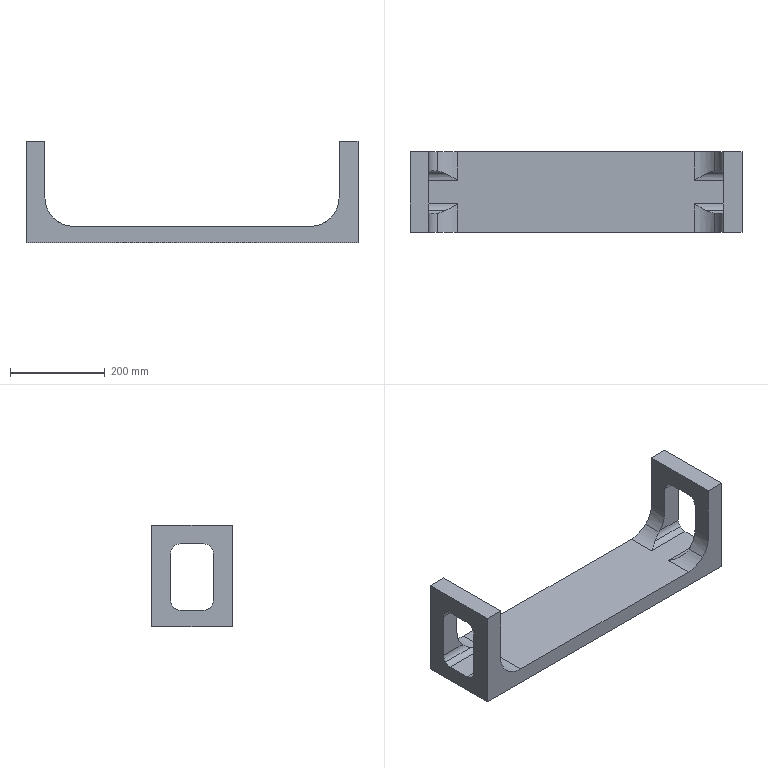Part | STEP file | ASND-0110-Forehead children guitar | 1 solid | 40 faces | box 700 x 170 x 215 mm | volume 5769786 mm3 | cylinder 24 | plane 16 | commonest cylinder face diameters 40 x16 120 x8